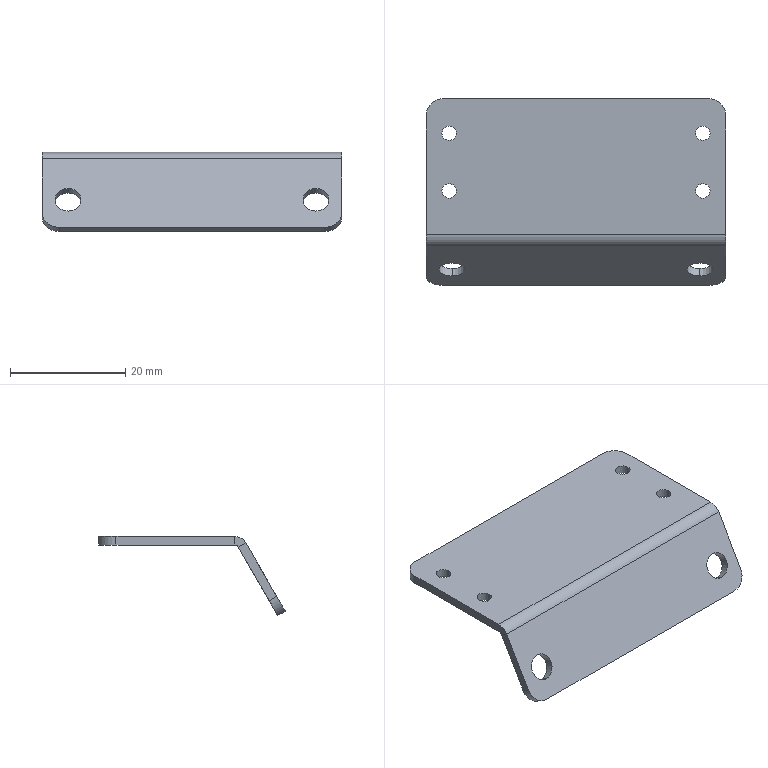Part | STEP file | 06-01-09 light source inclined plate (Default) | 1 solid | 30 faces | box 52 x 32.366 x 13.74 mm | volume 2941 mm3 | cylinder 18 | plane 12 | commonest cylinder face diameters 2.5 x8 4.5 x4 6 x4 1.473 x1 4.473 x1
STEP:
#1=CARTESIAN_POINT('',(21.5,-16.491,-6.279));
#2=VERTEX_POINT('',#1);
#3=CARTESIAN_POINT('',(21.5,-18.741,-10.176));
#4=VERTEX_POINT('',#3);
#5=CARTESIAN_POINT('',(21.5,-17.616,-8.227));
#6=DIRECTION('',(0.,-0.866,0.5));
#7=DIRECTION('',(0.,-0.5,-0.866));
#8=AXIS2_PLACEMENT_3D('',#5,#6,#7);
#9=CIRCLE('',#8,2.25);
#10=EDGE_CURVE('',#2,#4,#9,.T.);
#11=ORIENTED_EDGE('',*,*,#10,.T.);
#12=CARTESIAN_POINT('',(21.5,-17.442,-10.926));
#13=VERTEX_POINT('',#12);
#14=CARTESIAN_POINT('',(21.5,-26.102,-5.926));
#15=DIRECTION('',(0.,0.866,-0.5));
#16=VECTOR('',#15,1000.);
#17=LINE('',#14,#16);
#18=EDGE_CURVE('',#4,#13,#17,.T.);
#19=ORIENTED_EDGE('',*,*,#18,.T.);
#20=CARTESIAN_POINT('',(21.5,-15.192,-7.029));
#21=VERTEX_POINT('',#20);
#22=CARTESIAN_POINT('',(21.5,-16.317,-8.977));
#23=DIRECTION('',(0.,0.866,-0.5));
#24=DIRECTION('',(0.,0.5,0.866));
#25=AXIS2_PLACEMENT_3D('',#22,#23,#24);
#26=CIRCLE('',#25,2.25);
#27=EDGE_CURVE('',#13,#21,#26,.T.);
#28=ORIENTED_EDGE('',*,*,#27,.T.);
#29=CARTESIAN_POINT('',(21.5,-23.852,-2.029));
#30=DIRECTION('',(0.,0.866,-0.5));
#31=VECTOR('',#30,1000.);
#32=LINE('',#29,#31);
#33=EDGE_CURVE('',#2,#21,#32,.T.);
#34=ORIENTED_EDGE('',*,*,#33,.F.);
#35=EDGE_LOOP('',(#11,#19,#28,#34));
#36=FACE_OUTER_BOUND('',#35,.T.);
#37=CARTESIAN_POINT('',(21.5,-24.977,-3.977));
#38=DIRECTION('',(0.,0.866,-0.5));
#39=DIRECTION('',(0.,0.5,0.866));
#40=AXIS2_PLACEMENT_3D('',#37,#38,#39);
#41=CYLINDRICAL_SURFACE('',#40,2.25);
#42=ADVANCED_FACE('',(#36),#41,.F.);
#43=CARTESIAN_POINT('',(-21.5,-16.491,-6.279));
#44=VERTEX_POINT('',#43);
#45=CARTESIAN_POINT('',(-21.5,-18.741,-10.176));
#46=VERTEX_POINT('',#45);
#47=CARTESIAN_POINT('',(-21.5,-17.616,-8.227));
#48=DIRECTION('',(0.,-0.866,0.5));
#49=DIRECTION('',(0.,-0.5,-0.866));
#50=AXIS2_PLACEMENT_3D('',#47,#48,#49);
#51=CIRCLE('',#50,2.25);
#52=EDGE_CURVE('',#44,#46,#51,.T.);
#53=ORIENTED_EDGE('',*,*,#52,.T.);
#54=CARTESIAN_POINT('',(-21.5,-17.442,-10.926));
#55=VERTEX_POINT('',#54);
#56=CARTESIAN_POINT('',(-21.5,-26.102,-5.926));
#57=DIRECTION('',(0.,0.866,-0.5));
#58=VECTOR('',#57,1000.);
#59=LINE('',#56,#58);
#60=EDGE_CURVE('',#46,#55,#59,.T.);
#61=ORIENTED_EDGE('',*,*,#60,.T.);
#62=CARTESIAN_POINT('',(-21.5,-15.192,-7.029));
#63=VERTEX_POINT('',#62);
#64=CARTESIAN_POINT('',(-21.5,-16.317,-8.977));
#65=DIRECTION('',(0.,0.866,-0.5));
#66=DIRECTION('',(0.,0.5,0.866));
#67=AXIS2_PLACEMENT_3D('',#64,#65,#66);
#68=CIRCLE('',#67,2.25);
#69=EDGE_CURVE('',#55,#63,#68,.T.);
#70=ORIENTED_EDGE('',*,*,#69,.T.);
#71=CARTESIAN_POINT('',(-21.5,-23.852,-2.029));
#72=DIRECTION('',(0.,0.866,-0.5));
#73=VECTOR('',#72,1000.);
#74=LINE('',#71,#73);
#75=EDGE_CURVE('',#44,#63,#74,.T.);
#76=ORIENTED_EDGE('',*,*,#75,.F.);
#77=EDGE_LOOP('',(#53,#61,#70,#76));
#78=FACE_OUTER_BOUND('',#77,.T.);
#79=CARTESIAN_POINT('',(-21.5,-24.977,-3.977));
#80=DIRECTION('',(0.,0.866,-0.5));
#81=DIRECTION('',(0.,0.5,0.866));
#82=AXIS2_PLACEMENT_3D('',#79,#80,#81);
#83=CYLINDRICAL_SURFACE('',#82,2.25);
#84=ADVANCED_FACE('',(#78),#83,.F.);
#85=CARTESIAN_POINT('',(20.75,-4.,0.));
#86=VERTEX_POINT('',#85);
#87=CARTESIAN_POINT('',(23.25,-4.,0.));
#88=VERTEX_POINT('',#87);
#89=CARTESIAN_POINT('',(22.,-4.,0.));
#90=DIRECTION('',(0.,0.,1.));
#91=DIRECTION('',(1.,0.,0.));
#92=AXIS2_PLACEMENT_3D('',#89,#90,#91);
#93=CIRCLE('',#92,1.25);
#94=EDGE_CURVE('',#86,#88,#93,.T.);
#95=ORIENTED_EDGE('',*,*,#94,.T.);
#96=CARTESIAN_POINT('',(23.25,-4.,-1.5));
#97=VERTEX_POINT('',#96);
#98=CARTESIAN_POINT('',(23.25,-4.,-1.5));
#99=DIRECTION('',(0.,0.,-1.));
#100=VECTOR('',#99,1000.);
#101=LINE('',#98,#100);
#102=EDGE_CURVE('',#88,#97,#101,.T.);
#103=ORIENTED_EDGE('',*,*,#102,.T.);
#104=CARTESIAN_POINT('',(20.75,-4.,-1.5));
#105=VERTEX_POINT('',#104);
#106=CARTESIAN_POINT('',(22.,-4.,-1.5));
#107=DIRECTION('',(0.,0.,-1.));
#108=DIRECTION('',(-1.,0.,0.));
#109=AXIS2_PLACEMENT_3D('',#106,#107,#108);
#110=CIRCLE('',#109,1.25);
#111=EDGE_CURVE('',#97,#105,#110,.T.);
#112=ORIENTED_EDGE('',*,*,#111,.T.);
#113=CARTESIAN_POINT('',(20.75,-4.,-1.5));
#114=DIRECTION('',(0.,0.,-1.));
#115=VECTOR('',#114,1000.);
#116=LINE('',#113,#115);
#117=EDGE_CURVE('',#86,#105,#116,.T.);
#118=ORIENTED_EDGE('',*,*,#117,.F.);
#119=EDGE_LOOP('',(#95,#103,#112,#118));
#120=FACE_OUTER_BOUND('',#119,.T.);
#121=CARTESIAN_POINT('',(22.,-4.,-1.5));
#122=DIRECTION('',(0.,0.,-1.));
#123=DIRECTION('',(-1.,0.,0.));
#124=AXIS2_PLACEMENT_3D('',#121,#122,#123);
#125=CYLINDRICAL_SURFACE('',#124,1.25);
#126=ADVANCED_FACE('',(#120),#125,.F.);
#127=CARTESIAN_POINT('',(20.75,6.,0.));
#128=VERTEX_POINT('',#127);
#129=CARTESIAN_POINT('',(23.25,6.,0.));
#130=VERTEX_POINT('',#129);
#131=CARTESIAN_POINT('',(22.,6.,0.));
#132=DIRECTION('',(0.,0.,1.));
#133=DIRECTION('',(1.,0.,0.));
#134=AXIS2_PLACEMENT_3D('',#131,#132,#133);
#135=CIRCLE('',#134,1.25);
#136=EDGE_CURVE('',#128,#130,#135,.T.);
#137=ORIENTED_EDGE('',*,*,#136,.T.);
#138=CARTESIAN_POINT('',(23.25,6.,-1.5));
#139=VERTEX_POINT('',#138);
#140=CARTESIAN_POINT('',(23.25,6.,-1.5));
#141=DIRECTION('',(0.,0.,-1.));
#142=VECTOR('',#141,1000.);
#143=LINE('',#140,#142);
#144=EDGE_CURVE('',#130,#139,#143,.T.);
#145=ORIENTED_EDGE('',*,*,#144,.T.);
#146=CARTESIAN_POINT('',(20.75,6.,-1.5));
#147=VERTEX_POINT('',#146);
#148=CARTESIAN_POINT('',(22.,6.,-1.5));
#149=DIRECTION('',(0.,0.,-1.));
#150=DIRECTION('',(-1.,0.,0.));
#151=AXIS2_PLACEMENT_3D('',#148,#149,#150);
#152=CIRCLE('',#151,1.25);
#153=EDGE_CURVE('',#139,#147,#152,.T.);
#154=ORIENTED_EDGE('',*,*,#153,.T.);
#155=CARTESIAN_POINT('',(20.75,6.,-1.5));
#156=DIRECTION('',(0.,0.,-1.));
#157=VECTOR('',#156,1000.);
#158=LINE('',#155,#157);
#159=EDGE_CURVE('',#128,#147,#158,.T.);
#160=ORIENTED_EDGE('',*,*,#159,.F.);
#161=EDGE_LOOP('',(#137,#145,#154,#160));
#162=FACE_OUTER_BOUND('',#161,.T.);
#163=CARTESIAN_POINT('',(22.,6.,-1.5));
#164=DIRECTION('',(0.,0.,-1.));
#165=DIRECTION('',(-1.,0.,0.));
#166=AXIS2_PLACEMENT_3D('',#163,#164,#165);
#167=CYLINDRICAL_SURFACE('',#166,1.25);
#168=ADVANCED_FACE('',(#162),#167,.F.);
#169=CARTESIAN_POINT('',(-23.25,6.,0.));
#170=VERTEX_POINT('',#169);
#171=CARTESIAN_POINT('',(-20.75,6.,0.));
#172=VERTEX_POINT('',#171);
#173=CARTESIAN_POINT('',(-22.,6.,0.));
#174=DIRECTION('',(0.,0.,1.));
#175=DIRECTION('',(1.,0.,0.));
#176=AXIS2_PLACEMENT_3D('',#173,#174,#175);
#177=CIRCLE('',#176,1.25);
#178=EDGE_CURVE('',#170,#172,#177,.T.);
#179=ORIENTED_EDGE('',*,*,#178,.T.);
#180=CARTESIAN_POINT('',(-20.75,6.,-1.5));
#181=VERTEX_POINT('',#180);
#182=CARTESIAN_POINT('',(-20.75,6.,-1.5));
#183=DIRECTION('',(0.,0.,-1.));
#184=VECTOR('',#183,1000.);
#185=LINE('',#182,#184);
#186=EDGE_CURVE('',#172,#181,#185,.T.);
#187=ORIENTED_EDGE('',*,*,#186,.T.);
#188=CARTESIAN_POINT('',(-23.25,6.,-1.5));
#189=VERTEX_POINT('',#188);
#190=CARTESIAN_POINT('',(-22.,6.,-1.5));
#191=DIRECTION('',(0.,0.,-1.));
#192=DIRECTION('',(-1.,0.,0.));
#193=AXIS2_PLACEMENT_3D('',#190,#191,#192);
#194=CIRCLE('',#193,1.25);
#195=EDGE_CURVE('',#181,#189,#194,.T.);
#196=ORIENTED_EDGE('',*,*,#195,.T.);
#197=CARTESIAN_POINT('',(-23.25,6.,-1.5));
#198=DIRECTION('',(0.,0.,-1.));
#199=VECTOR('',#198,1000.);
#200=LINE('',#197,#199);
#201=EDGE_CURVE('',#170,#189,#200,.T.);
#202=ORIENTED_EDGE('',*,*,#201,.F.);
#203=EDGE_LOOP('',(#179,#187,#196,#202));
#204=FACE_OUTER_BOUND('',#203,.T.);
#205=CARTESIAN_POINT('',(-22.,6.,-1.5));
#206=DIRECTION('',(0.,0.,-1.));
#207=DIRECTION('',(-1.,0.,0.));
#208=AXIS2_PLACEMENT_3D('',#205,#206,#207);
#209=CYLINDRICAL_SURFACE('',#208,1.25);
#210=ADVANCED_FACE('',(#204),#209,.F.);
#211=CARTESIAN_POINT('',(-23.25,-4.,0.));
#212=VERTEX_POINT('',#211);
#213=CARTESIAN_POINT('',(-20.75,-4.,0.));
#214=VERTEX_POINT('',#213);
#215=CARTESIAN_POINT('',(-22.,-4.,0.));
#216=DIRECTION('',(0.,0.,1.));
#217=DIRECTION('',(1.,0.,0.));
#218=AXIS2_PLACEMENT_3D('',#215,#216,#217);
#219=CIRCLE('',#218,1.25);
#220=EDGE_CURVE('',#212,#214,#219,.T.);
#221=ORIENTED_EDGE('',*,*,#220,.T.);
#222=CARTESIAN_POINT('',(-20.75,-4.,-1.5));
#223=VERTEX_POINT('',#222);
#224=CARTESIAN_POINT('',(-20.75,-4.,-1.5));
#225=DIRECTION('',(0.,0.,-1.));
#226=VECTOR('',#225,1000.);
#227=LINE('',#224,#226);
#228=EDGE_CURVE('',#214,#223,#227,.T.);
#229=ORIENTED_EDGE('',*,*,#228,.T.);
#230=CARTESIAN_POINT('',(-23.25,-4.,-1.5));
#231=VERTEX_POINT('',#230);
#232=CARTESIAN_POINT('',(-22.,-4.,-1.5));
#233=DIRECTION('',(0.,0.,-1.));
#234=DIRECTION('',(-1.,0.,0.));
#235=AXIS2_PLACEMENT_3D('',#232,#233,#234);
#236=CIRCLE('',#235,1.25);
#237=EDGE_CURVE('',#223,#231,#236,.T.);
#238=ORIENTED_EDGE('',*,*,#237,.T.);
#239=CARTESIAN_POINT('',(-23.25,-4.,-1.5));
#240=DIRECTION('',(0.,0.,-1.));
#241=VECTOR('',#240,1000.);
#242=LINE('',#239,#241);
#243=EDGE_CURVE('',#212,#231,#242,.T.);
#244=ORIENTED_EDGE('',*,*,#243,.F.);
#245=EDGE_LOOP('',(#221,#229,#238,#244));
#246=FACE_OUTER_BOUND('',#245,.T.);
#247=CARTESIAN_POINT('',(-22.,-4.,-1.5));
#248=DIRECTION('',(0.,0.,-1.));
#249=DIRECTION('',(-1.,0.,0.));
#250=AXIS2_PLACEMENT_3D('',#247,#248,#249);
#251=CYLINDRICAL_SURFACE('',#250,1.25);
#252=ADVANCED_FACE('',(#246),#251,.F.);
#253=CARTESIAN_POINT('',(-26.,9.,0.));
#254=VERTEX_POINT('',#253);
#255=CARTESIAN_POINT('',(-26.,-11.575,0.));
#256=VERTEX_POINT('',#255);
#257=CARTESIAN_POINT('',(-26.,12.,0.));
#258=DIRECTION('',(0.,-1.,0.));
#259=VECTOR('',#258,1000.);
#260=LINE('',#257,#259);
#261=EDGE_CURVE('',#254,#256,#260,.T.);
#262=ORIENTED_EDGE('',*,*,#261,.F.);
#263=CARTESIAN_POINT('',(-26.,9.,-1.5));
#264=VERTEX_POINT('',#263);
#265=CARTESIAN_POINT('',(-26.,9.,-1.5));
#266=DIRECTION('',(0.,0.,-1.));
#267=VECTOR('',#266,1000.);
#268=LINE('',#265,#267);
#269=EDGE_CURVE('',#254,#264,#268,.T.);
#270=ORIENTED_EDGE('',*,*,#269,.T.);
#271=CARTESIAN_POINT('',(-26.,-11.575,-1.5));
#272=VERTEX_POINT('',#271);
#273=CARTESIAN_POINT('',(-26.,12.,-1.5));
#274=DIRECTION('',(0.,-1.,0.));
#275=VECTOR('',#274,1000.);
#276=LINE('',#273,#275);
#277=EDGE_CURVE('',#264,#272,#276,.T.);
#278=ORIENTED_EDGE('',*,*,#277,.T.);
#279=CARTESIAN_POINT('',(-26.,-11.575,-1.5));
#280=DIRECTION('',(0.,0.,1.));
#281=VECTOR('',#280,1000.);
#282=LINE('',#279,#281);
#283=EDGE_CURVE('',#272,#256,#282,.T.);
#284=ORIENTED_EDGE('',*,*,#283,.T.);
#285=EDGE_LOOP('',(#262,#270,#278,#284));
#286=FACE_OUTER_BOUND('',#285,.T.);
#287=CARTESIAN_POINT('',(-26.,12.,-1.5));
#288=DIRECTION('',(-1.,0.,0.));
#289=DIRECTION('',(0.,-1.,0.));
#290=AXIS2_PLACEMENT_3D('',#287,#288,#289);
#291=PLANE('',#290);
#292=ADVANCED_FACE('',(#286),#291,.T.);
#293=CARTESIAN_POINT('',(22.,-4.,-1.5));
#294=DIRECTION('',(0.,0.,-1.));
#295=DIRECTION('',(-1.,0.,0.));
#296=AXIS2_PLACEMENT_3D('',#293,#294,#295);
#297=CIRCLE('',#296,1.25);
#298=EDGE_CURVE('',#105,#97,#297,.T.);
#299=ORIENTED_EDGE('',*,*,#298,.F.);
#300=ORIENTED_EDGE('',*,*,#111,.F.);
#301=EDGE_LOOP('',(#299,#300));
#302=FACE_BOUND('',#301,.T.);
#303=CARTESIAN_POINT('',(22.,6.,-1.5));
#304=DIRECTION('',(0.,0.,-1.));
#305=DIRECTION('',(-1.,0.,0.));
#306=AXIS2_PLACEMENT_3D('',#303,#304,#305);
#307=CIRCLE('',#306,1.25);
#308=EDGE_CURVE('',#147,#139,#307,.T.);
#309=ORIENTED_EDGE('',*,*,#308,.F.);
#310=ORIENTED_EDGE('',*,*,#153,.F.);
#311=EDGE_LOOP('',(#309,#310));
#312=FACE_BOUND('',#311,.T.);
#313=CARTESIAN_POINT('',(-22.,6.,-1.5));
#314=DIRECTION('',(0.,0.,-1.));
#315=DIRECTION('',(-1.,0.,0.));
#316=AXIS2_PLACEMENT_3D('',#313,#314,#315);
#317=CIRCLE('',#316,1.25);
#318=EDGE_CURVE('',#189,#181,#317,.T.);
#319=ORIENTED_EDGE('',*,*,#318,.F.);
#320=ORIENTED_EDGE('',*,*,#195,.F.);
#321=EDGE_LOOP('',(#319,#320));
#322=FACE_BOUND('',#321,.T.);
#323=CARTESIAN_POINT('',(-22.,-4.,-1.5));
#324=DIRECTION('',(0.,0.,-1.));
#325=DIRECTION('',(-1.,0.,0.));
#326=AXIS2_PLACEMENT_3D('',#323,#324,#325);
#327=CIRCLE('',#326,1.25);
#328=EDGE_CURVE('',#231,#223,#327,.T.);
#329=ORIENTED_EDGE('',*,*,#328,.F.);
#330=ORIENTED_EDGE('',*,*,#237,.F.);
#331=EDGE_LOOP('',(#329,#330));
#332=FACE_BOUND('',#331,.T.);
#333=ORIENTED_EDGE('',*,*,#277,.F.);
#334=CARTESIAN_POINT('',(-23.,12.,-1.5));
#335=VERTEX_POINT('',#334);
#336=CARTESIAN_POINT('',(-23.,9.,-1.5));
#337=DIRECTION('',(0.,0.,-1.));
#338=DIRECTION('',(1.,0.,0.));
#339=AXIS2_PLACEMENT_3D('',#336,#337,#338);
#340=CIRCLE('',#339,3.);
#341=EDGE_CURVE('',#264,#335,#340,.T.);
#342=ORIENTED_EDGE('',*,*,#341,.T.);
#343=CARTESIAN_POINT('',(23.,12.,-1.5));
#344=VERTEX_POINT('',#343);
#345=CARTESIAN_POINT('',(-26.,12.,-1.5));
#346=DIRECTION('',(-1.,0.,0.));
#347=VECTOR('',#346,1000.);
#348=LINE('',#345,#347);
#349=EDGE_CURVE('',#344,#335,#348,.T.);
#350=ORIENTED_EDGE('',*,*,#349,.F.);
#351=CARTESIAN_POINT('',(26.,9.,-1.5));
#352=VERTEX_POINT('',#351);
#353=CARTESIAN_POINT('',(23.,9.,-1.5));
#354=DIRECTION('',(0.,0.,-1.));
#355=DIRECTION('',(1.,0.,0.));
#356=AXIS2_PLACEMENT_3D('',#353,#354,#355);
#357=CIRCLE('',#356,3.);
#358=EDGE_CURVE('',#344,#352,#357,.T.);
#359=ORIENTED_EDGE('',*,*,#358,.T.);
#360=CARTESIAN_POINT('',(26.,-11.575,-1.5));
#361=VERTEX_POINT('',#360);
#362=CARTESIAN_POINT('',(26.,12.,-1.5));
#363=DIRECTION('',(0.,1.,0.));
#364=VECTOR('',#363,1000.);
#365=LINE('',#362,#364);
#366=EDGE_CURVE('',#361,#352,#365,.T.);
#367=ORIENTED_EDGE('',*,*,#366,.F.);
#368=CARTESIAN_POINT('',(-26.,-11.575,-1.5));
#369=DIRECTION('',(1.,0.,0.));
#370=VECTOR('',#369,1000.);
#371=LINE('',#368,#370);
#372=EDGE_CURVE('',#272,#361,#371,.T.);
#373=ORIENTED_EDGE('',*,*,#372,.F.);
#374=EDGE_LOOP('',(#333,#342,#350,#359,#367,#373));
#375=FACE_OUTER_BOUND('',#374,.T.);
#376=CARTESIAN_POINT('',(26.,-12.,-1.5));
#377=DIRECTION('',(0.,0.,1.));
#378=DIRECTION('',(1.,0.,0.));
#379=AXIS2_PLACEMENT_3D('',#376,#377,#378);
#380=PLANE('',#379);
#381=ADVANCED_FACE('',(#302,#312,#322,#332,#375),#380,.F.);
#382=ORIENTED_EDGE('',*,*,#94,.F.);
#383=CARTESIAN_POINT('',(22.,-4.,0.));
#384=DIRECTION('',(0.,0.,1.));
#385=DIRECTION('',(1.,0.,0.));
#386=AXIS2_PLACEMENT_3D('',#383,#384,#385);
#387=CIRCLE('',#386,1.25);
#388=EDGE_CURVE('',#88,#86,#387,.T.);
#389=ORIENTED_EDGE('',*,*,#388,.F.);
#390=EDGE_LOOP('',(#382,#389));
#391=FACE_BOUND('',#390,.T.);
#392=ORIENTED_EDGE('',*,*,#136,.F.);
#393=CARTESIAN_POINT('',(22.,6.,0.));
#394=DIRECTION('',(0.,0.,1.));
#395=DIRECTION('',(1.,0.,0.));
#396=AXIS2_PLACEMENT_3D('',#393,#394,#395);
#397=CIRCLE('',#396,1.25);
#398=EDGE_CURVE('',#130,#128,#397,.T.);
#399=ORIENTED_EDGE('',*,*,#398,.F.);
#400=EDGE_LOOP('',(#392,#399));
#401=FACE_BOUND('',#400,.T.);
#402=ORIENTED_EDGE('',*,*,#178,.F.);
#403=CARTESIAN_POINT('',(-22.,6.,0.));
#404=DIRECTION('',(0.,0.,1.));
#405=DIRECTION('',(1.,0.,0.));
#406=AXIS2_PLACEMENT_3D('',#403,#404,#405);
#407=CIRCLE('',#406,1.25);
#408=EDGE_CURVE('',#172,#170,#407,.T.);
#409=ORIENTED_EDGE('',*,*,#408,.F.);
#410=EDGE_LOOP('',(#402,#409));
#411=FACE_BOUND('',#410,.T.);
#412=ORIENTED_EDGE('',*,*,#220,.F.);
#413=CARTESIAN_POINT('',(-22.,-4.,0.));
#414=DIRECTION('',(0.,0.,1.));
#415=DIRECTION('',(1.,0.,0.));
#416=AXIS2_PLACEMENT_3D('',#413,#414,#415);
#417=CIRCLE('',#416,1.25);
#418=EDGE_CURVE('',#214,#212,#417,.T.);
#419=ORIENTED_EDGE('',*,*,#418,.F.);
#420=EDGE_LOOP('',(#412,#419));
#421=FACE_BOUND('',#420,.T.);
#422=CARTESIAN_POINT('',(23.,12.,0.));
#423=VERTEX_POINT('',#422);
#424=CARTESIAN_POINT('',(-23.,12.,0.));
#425=VERTEX_POINT('',#424);
#426=CARTESIAN_POINT('',(-26.,12.,0.));
#427=DIRECTION('',(-1.,0.,0.));
#428=VECTOR('',#427,1000.);
#429=LINE('',#426,#428);
#430=EDGE_CURVE('',#423,#425,#429,.T.);
#431=ORIENTED_EDGE('',*,*,#430,.T.);
#432=CARTESIAN_POINT('',(-23.,9.,0.));
#433=DIRECTION('',(0.,0.,1.));
#434=DIRECTION('',(1.,0.,0.));
#435=AXIS2_PLACEMENT_3D('',#432,#433,#434);
#436=CIRCLE('',#435,3.);
#437=EDGE_CURVE('',#425,#254,#436,.T.);
#438=ORIENTED_EDGE('',*,*,#437,.T.);
#439=ORIENTED_EDGE('',*,*,#261,.T.);
#440=CARTESIAN_POINT('',(26.,-11.575,0.));
#441=VERTEX_POINT('',#440);
#442=CARTESIAN_POINT('',(-26.,-11.575,0.));
#443=DIRECTION('',(1.,0.,0.));
#444=VECTOR('',#443,1000.);
#445=LINE('',#442,#444);
#446=EDGE_CURVE('',#256,#441,#445,.T.);
#447=ORIENTED_EDGE('',*,*,#446,.T.);
#448=CARTESIAN_POINT('',(26.,9.,0.));
#449=VERTEX_POINT('',#448);
#450=CARTESIAN_POINT('',(26.,12.,0.));
#451=DIRECTION('',(0.,1.,0.));
#452=VECTOR('',#451,1000.);
#453=LINE('',#450,#452);
#454=EDGE_CURVE('',#441,#449,#453,.T.);
#455=ORIENTED_EDGE('',*,*,#454,.T.);
#456=CARTESIAN_POINT('',(23.,9.,0.));
#457=DIRECTION('',(0.,0.,1.));
#458=DIRECTION('',(1.,0.,0.));
#459=AXIS2_PLACEMENT_3D('',#456,#457,#458);
#460=CIRCLE('',#459,3.);
#461=EDGE_CURVE('',#449,#423,#460,.T.);
#462=ORIENTED_EDGE('',*,*,#461,.T.);
#463=EDGE_LOOP('',(#431,#438,#439,#447,#455,#462));
#464=FACE_OUTER_BOUND('',#463,.T.);
#465=CARTESIAN_POINT('',(26.,-12.,0.));
#466=DIRECTION('',(0.,0.,1.));
#467=DIRECTION('',(1.,0.,0.));
#468=AXIS2_PLACEMENT_3D('',#465,#466,#467);
#469=PLANE('',#468);
#470=ADVANCED_FACE('',(#391,#401,#411,#421,#464),#469,.T.);
#471=ORIENTED_EDGE('',*,*,#366,.T.);
#472=CARTESIAN_POINT('',(26.,9.,-1.5));
#473=DIRECTION('',(0.,0.,1.));
#474=VECTOR('',#473,1000.);
#475=LINE('',#472,#474);
#476=EDGE_CURVE('',#352,#449,#475,.T.);
#477=ORIENTED_EDGE('',*,*,#476,.T.);
#478=ORIENTED_EDGE('',*,*,#454,.F.);
#479=CARTESIAN_POINT('',(26.,-11.575,-1.5));
#480=DIRECTION('',(0.,0.,1.));
#481=VECTOR('',#480,1000.);
#482=LINE('',#479,#481);
#483=EDGE_CURVE('',#361,#441,#482,.T.);
#484=ORIENTED_EDGE('',*,*,#483,.F.);
#485=EDGE_LOOP('',(#471,#477,#478,#484));
#486=FACE_OUTER_BOUND('',#485,.T.);
#487=CARTESIAN_POINT('',(26.,12.,-1.5));
#488=DIRECTION('',(1.,0.,0.));
#489=DIRECTION('',(0.,0.,-1.));
#490=AXIS2_PLACEMENT_3D('',#487,#488,#489);
#491=PLANE('',#490);
#492=ADVANCED_FACE('',(#486),#491,.T.);
#493=ORIENTED_EDGE('',*,*,#349,.T.);
#494=CARTESIAN_POINT('',(-23.,12.,-1.5));
#495=DIRECTION('',(0.,0.,1.));
#496=VECTOR('',#495,1000.);
#497=LINE('',#494,#496);
#498=EDGE_CURVE('',#335,#425,#497,.T.);
#499=ORIENTED_EDGE('',*,*,#498,.T.);
#500=ORIENTED_EDGE('',*,*,#430,.F.);
#501=CARTESIAN_POINT('',(23.,12.,-1.5));
#502=DIRECTION('',(0.,0.,-1.));
#503=VECTOR('',#502,1000.);
#504=LINE('',#501,#503);
#505=EDGE_CURVE('',#423,#344,#504,.T.);
#506=ORIENTED_EDGE('',*,*,#505,.T.);
#507=EDGE_LOOP('',(#493,#499,#500,#506));
#508=FACE_OUTER_BOUND('',#507,.T.);
#509=CARTESIAN_POINT('',(-26.,12.,-1.5));
#510=DIRECTION('',(0.,1.,0.));
#511=DIRECTION('',(0.,0.,1.));
#512=AXIS2_PLACEMENT_3D('',#509,#510,#511);
#513=PLANE('',#512);
#514=ADVANCED_FACE('',(#508),#513,.T.);
#515=CARTESIAN_POINT('',(26.,-12.213,-1.868));
#516=VERTEX_POINT('',#515);
#517=CARTESIAN_POINT('',(26.,-13.512,-1.118));
#518=VERTEX_POINT('',#517);
#519=CARTESIAN_POINT('',(26.,-12.213,-1.868));
#520=DIRECTION('',(0.,-0.866,0.5));
#521=VECTOR('',#520,1000.);
#522=LINE('',#519,#521);
#523=EDGE_CURVE('',#516,#518,#522,.T.);
#524=ORIENTED_EDGE('',*,*,#523,.F.);
#525=CARTESIAN_POINT('',(26.,-11.575,-2.237));
#526=DIRECTION('',(1.,0.,0.));
#527=DIRECTION('',(0.,0.,1.));
#528=AXIS2_PLACEMENT_3D('',#525,#526,#527);
#529=CIRCLE('',#528,0.7366);
#530=EDGE_CURVE('',#361,#516,#529,.T.);
#531=ORIENTED_EDGE('',*,*,#530,.F.);
#532=ORIENTED_EDGE('',*,*,#483,.T.);
#533=CARTESIAN_POINT('',(26.,-11.575,-2.237));
#534=DIRECTION('',(1.,0.,0.));
#535=DIRECTION('',(0.,0.,1.));
#536=AXIS2_PLACEMENT_3D('',#533,#534,#535);
#537=CIRCLE('',#536,2.237);
#538=EDGE_CURVE('',#441,#518,#537,.T.);
#539=ORIENTED_EDGE('',*,*,#538,.T.);
#540=EDGE_LOOP('',(#524,#531,#532,#539));
#541=FACE_OUTER_BOUND('',#540,.T.);
#542=CARTESIAN_POINT('',(26.,-11.575,-2.237));
#543=DIRECTION('',(1.,0.,0.));
#544=DIRECTION('',(0.,0.,-1.));
#545=AXIS2_PLACEMENT_3D('',#542,#543,#544);
#546=PLANE('',#545);
#547=ADVANCED_FACE('',(#541),#546,.T.);
#548=CARTESIAN_POINT('',(-26.,-12.213,-1.868));
#549=VERTEX_POINT('',#548);
#550=CARTESIAN_POINT('',(-26.,-11.575,-2.237));
#551=DIRECTION('',(-1.,0.,0.));
#552=DIRECTION('',(0.,0.,1.));
#553=AXIS2_PLACEMENT_3D('',#550,#551,#552);
#554=CIRCLE('',#553,0.7366);
#555=EDGE_CURVE('',#549,#272,#554,.T.);
#556=ORIENTED_EDGE('',*,*,#555,.F.);
#557=CARTESIAN_POINT('',(-26.,-13.512,-1.118));
#558=VERTEX_POINT('',#557);
#559=CARTESIAN_POINT('',(-26.,-12.213,-1.868));
#560=DIRECTION('',(0.,-0.866,0.5));
#561=VECTOR('',#560,1000.);
#562=LINE('',#559,#561);
#563=EDGE_CURVE('',#549,#558,#562,.T.);
#564=ORIENTED_EDGE('',*,*,#563,.T.);
#565=CARTESIAN_POINT('',(-26.,-11.575,-2.237));
#566=DIRECTION('',(-1.,0.,0.));
#567=DIRECTION('',(0.,0.,1.));
#568=AXIS2_PLACEMENT_3D('',#565,#566,#567);
#569=CIRCLE('',#568,2.237);
#570=EDGE_CURVE('',#558,#256,#569,.T.);
#571=ORIENTED_EDGE('',*,*,#570,.T.);
#572=ORIENTED_EDGE('',*,*,#283,.F.);
#573=EDGE_LOOP('',(#556,#564,#571,#572));
#574=FACE_OUTER_BOUND('',#573,.T.);
#575=CARTESIAN_POINT('',(-26.,-11.575,-2.237));
#576=DIRECTION('',(1.,0.,0.));
#577=DIRECTION('',(0.,0.,-1.));
#578=AXIS2_PLACEMENT_3D('',#575,#576,#577);
#579=PLANE('',#578);
#580=ADVANCED_FACE('',(#574),#579,.F.);
#581=ORIENTED_EDGE('',*,*,#446,.F.);
#582=ORIENTED_EDGE('',*,*,#570,.F.);
#583=CARTESIAN_POINT('',(-26.,-13.512,-1.118));
#584=DIRECTION('',(-1.,0.,0.));
#585=VECTOR('',#584,1000.);
#586=LINE('',#583,#585);
#587=EDGE_CURVE('',#518,#558,#586,.T.);
#588=ORIENTED_EDGE('',*,*,#587,.F.);
#589=ORIENTED_EDGE('',*,*,#538,.F.);
#590=EDGE_LOOP('',(#581,#582,#588,#589));
#591=FACE_OUTER_BOUND('',#590,.T.);
#592=CARTESIAN_POINT('',(-26.,-11.575,-2.237));
#593=DIRECTION('',(-1.,0.,0.));
#594=DIRECTION('',(0.,-0.866,0.5));
#595=AXIS2_PLACEMENT_3D('',#592,#593,#594);
#596=CYLINDRICAL_SURFACE('',#595,2.237);
#597=ADVANCED_FACE('',(#591),#596,.T.);
#598=ORIENTED_EDGE('',*,*,#372,.T.);
#599=ORIENTED_EDGE('',*,*,#530,.T.);
#600=CARTESIAN_POINT('',(26.,-12.213,-1.868));
#601=DIRECTION('',(-1.,0.,0.));
#602=VECTOR('',#601,1000.);
#603=LINE('',#600,#602);
#604=EDGE_CURVE('',#516,#549,#603,.T.);
#605=ORIENTED_EDGE('',*,*,#604,.T.);
#606=ORIENTED_EDGE('',*,*,#555,.T.);
#607=EDGE_LOOP('',(#598,#599,#605,#606));
#608=FACE_OUTER_BOUND('',#607,.T.);
#609=CARTESIAN_POINT('',(-26.,-11.575,-2.237));
#610=DIRECTION('',(-1.,0.,0.));
#611=DIRECTION('',(0.,-0.866,0.5));
#612=AXIS2_PLACEMENT_3D('',#609,#610,#611);
#613=CYLINDRICAL_SURFACE('',#612,0.7366);
#614=ADVANCED_FACE('',(#608),#613,.F.);
#615=CARTESIAN_POINT('',(-26.,-17.567,-11.142));
#616=VERTEX_POINT('',#615);
#617=CARTESIAN_POINT('',(-26.,-12.,-1.5));
#618=DIRECTION('',(0.,0.5,0.866));
#619=VECTOR('',#618,1000.);
#620=LINE('',#617,#619);
#621=EDGE_CURVE('',#616,#549,#620,.T.);
#622=ORIENTED_EDGE('',*,*,#621,.F.);
#623=CARTESIAN_POINT('',(-26.,-18.866,-10.392));
#624=VERTEX_POINT('',#623);
#625=CARTESIAN_POINT('',(-26.,-18.866,-10.392));
#626=DIRECTION('',(0.,-0.866,0.5));
#627=VECTOR('',#626,1000.);
#628=LINE('',#625,#627);
#629=EDGE_CURVE('',#616,#624,#628,.T.);
#630=ORIENTED_EDGE('',*,*,#629,.T.);
#631=CARTESIAN_POINT('',(-26.,-13.299,-0.75));
#632=DIRECTION('',(0.,0.5,0.866));
#633=VECTOR('',#632,1000.);
#634=LINE('',#631,#633);
#635=EDGE_CURVE('',#624,#558,#634,.T.);
#636=ORIENTED_EDGE('',*,*,#635,.T.);
#637=ORIENTED_EDGE('',*,*,#563,.F.);
#638=EDGE_LOOP('',(#622,#630,#636,#637));
#639=FACE_OUTER_BOUND('',#638,.T.);
#640=CARTESIAN_POINT('',(-26.,-13.299,-0.75));
#641=DIRECTION('',(-1.,0.,0.));
#642=DIRECTION('',(0.,0.,1.));
#643=AXIS2_PLACEMENT_3D('',#640,#641,#642);
#644=PLANE('',#643);
#645=ADVANCED_FACE('',(#639),#644,.T.);
#646=CARTESIAN_POINT('',(26.,-18.866,-10.392));
#647=VERTEX_POINT('',#646);
#648=CARTESIAN_POINT('',(26.,-20.366,-12.99));
#649=DIRECTION('',(0.,-0.5,-0.866));
#650=VECTOR('',#649,1000.);
#651=LINE('',#648,#650);
#652=EDGE_CURVE('',#518,#647,#651,.T.);
#653=ORIENTED_EDGE('',*,*,#652,.T.);
#654=CARTESIAN_POINT('',(26.,-17.567,-11.142));
#655=VERTEX_POINT('',#654);
#656=CARTESIAN_POINT('',(26.,-18.866,-10.392));
#657=DIRECTION('',(0.,0.866,-0.5));
#658=VECTOR('',#657,1000.);
#659=LINE('',#656,#658);
#660=EDGE_CURVE('',#647,#655,#659,.T.);
#661=ORIENTED_EDGE('',*,*,#660,.T.);
#662=CARTESIAN_POINT('',(26.,-19.067,-13.74));
#663=DIRECTION('',(0.,-0.5,-0.866));
#664=VECTOR('',#663,1000.);
#665=LINE('',#662,#664);
#666=EDGE_CURVE('',#516,#655,#665,.T.);
#667=ORIENTED_EDGE('',*,*,#666,.F.);
#668=ORIENTED_EDGE('',*,*,#523,.T.);
#669=EDGE_LOOP('',(#653,#661,#667,#668));
#670=FACE_OUTER_BOUND('',#669,.T.);
#671=CARTESIAN_POINT('',(26.,-20.366,-12.99));
#672=DIRECTION('',(1.,0.,0.));
#673=DIRECTION('',(0.,0.,-1.));
#674=AXIS2_PLACEMENT_3D('',#671,#672,#673);
#675=PLANE('',#674);
#676=ADVANCED_FACE('',(#670),#675,.T.);
#677=ORIENTED_EDGE('',*,*,#10,.F.);
#678=CARTESIAN_POINT('',(21.5,-17.616,-8.227));
#679=DIRECTION('',(0.,-0.866,0.5));
#680=DIRECTION('',(0.,-0.5,-0.866));
#681=AXIS2_PLACEMENT_3D('',#678,#679,#680);
#682=CIRCLE('',#681,2.25);
#683=EDGE_CURVE('',#4,#2,#682,.T.);
#684=ORIENTED_EDGE('',*,*,#683,.F.);
#685=EDGE_LOOP('',(#677,#684));
#686=FACE_BOUND('',#685,.T.);
#687=ORIENTED_EDGE('',*,*,#52,.F.);
#688=CARTESIAN_POINT('',(-21.5,-17.616,-8.227));
#689=DIRECTION('',(0.,-0.866,0.5));
#690=DIRECTION('',(0.,-0.5,-0.866));
#691=AXIS2_PLACEMENT_3D('',#688,#689,#690);
#692=CIRCLE('',#691,2.25);
#693=EDGE_CURVE('',#46,#44,#692,.T.);
#694=ORIENTED_EDGE('',*,*,#693,.F.);
#695=EDGE_LOOP('',(#687,#694));
#696=FACE_BOUND('',#695,.T.);
#697=ORIENTED_EDGE('',*,*,#635,.F.);
#698=CARTESIAN_POINT('',(-23.,-20.366,-12.99));
#699=VERTEX_POINT('',#698);
#700=CARTESIAN_POINT('',(-23.,-18.866,-10.392));
#701=DIRECTION('',(0.,-0.866,0.5));
#702=DIRECTION('',(0.,-0.5,-0.866));
#703=AXIS2_PLACEMENT_3D('',#700,#701,#702);
#704=CIRCLE('',#703,3.);
#705=EDGE_CURVE('',#624,#699,#704,.T.);
#706=ORIENTED_EDGE('',*,*,#705,.T.);
#707=CARTESIAN_POINT('',(23.,-20.366,-12.99));
#708=VERTEX_POINT('',#707);
#709=CARTESIAN_POINT('',(-26.,-20.366,-12.99));
#710=DIRECTION('',(-1.,0.,0.));
#711=VECTOR('',#710,1000.);
#712=LINE('',#709,#711);
#713=EDGE_CURVE('',#708,#699,#712,.T.);
#714=ORIENTED_EDGE('',*,*,#713,.F.);
#715=CARTESIAN_POINT('',(23.,-18.866,-10.392));
#716=DIRECTION('',(0.,-0.866,0.5));
#717=DIRECTION('',(0.,-0.5,-0.866));
#718=AXIS2_PLACEMENT_3D('',#715,#716,#717);
#719=CIRCLE('',#718,3.);
#720=EDGE_CURVE('',#708,#647,#719,.T.);
#721=ORIENTED_EDGE('',*,*,#720,.T.);
#722=ORIENTED_EDGE('',*,*,#652,.F.);
#723=ORIENTED_EDGE('',*,*,#587,.T.);
#724=EDGE_LOOP('',(#697,#706,#714,#721,#722,#723));
#725=FACE_OUTER_BOUND('',#724,.T.);
#726=CARTESIAN_POINT('',(-26.,-13.299,-0.75));
#727=DIRECTION('',(0.,-0.866,0.5));
#728=DIRECTION('',(0.,-0.5,-0.866));
#729=AXIS2_PLACEMENT_3D('',#726,#727,#728);
#730=PLANE('',#729);
#731=ADVANCED_FACE('',(#686,#696,#725),#730,.T.);
#732=CARTESIAN_POINT('',(21.5,-16.317,-8.977));
#733=DIRECTION('',(0.,0.866,-0.5));
#734=DIRECTION('',(0.,0.5,0.866));
#735=AXIS2_PLACEMENT_3D('',#732,#733,#734);
#736=CIRCLE('',#735,2.25);
#737=EDGE_CURVE('',#21,#13,#736,.T.);
#738=ORIENTED_EDGE('',*,*,#737,.F.);
#739=ORIENTED_EDGE('',*,*,#27,.F.);
#740=EDGE_LOOP('',(#738,#739));
#741=FACE_BOUND('',#740,.T.);
#742=CARTESIAN_POINT('',(-21.5,-16.317,-8.977));
#743=DIRECTION('',(0.,0.866,-0.5));
#744=DIRECTION('',(0.,0.5,0.866));
#745=AXIS2_PLACEMENT_3D('',#742,#743,#744);
#746=CIRCLE('',#745,2.25);
#747=EDGE_CURVE('',#63,#55,#746,.T.);
#748=ORIENTED_EDGE('',*,*,#747,.F.);
#749=ORIENTED_EDGE('',*,*,#69,.F.);
#750=EDGE_LOOP('',(#748,#749));
#751=FACE_BOUND('',#750,.T.);
#752=CARTESIAN_POINT('',(23.,-19.067,-13.74));
#753=VERTEX_POINT('',#752);
#754=CARTESIAN_POINT('',(-23.,-19.067,-13.74));
#755=VERTEX_POINT('',#754);
#756=CARTESIAN_POINT('',(-26.,-19.067,-13.74));
#757=DIRECTION('',(-1.,0.,0.));
#758=VECTOR('',#757,1000.);
#759=LINE('',#756,#758);
#760=EDGE_CURVE('',#753,#755,#759,.T.);
#761=ORIENTED_EDGE('',*,*,#760,.T.);
#762=CARTESIAN_POINT('',(-23.,-17.567,-11.142));
#763=DIRECTION('',(0.,0.866,-0.5));
#764=DIRECTION('',(0.,-0.5,-0.866));
#765=AXIS2_PLACEMENT_3D('',#762,#763,#764);
#766=CIRCLE('',#765,3.);
#767=EDGE_CURVE('',#755,#616,#766,.T.);
#768=ORIENTED_EDGE('',*,*,#767,.T.);
#769=ORIENTED_EDGE('',*,*,#621,.T.);
#770=ORIENTED_EDGE('',*,*,#604,.F.);
#771=ORIENTED_EDGE('',*,*,#666,.T.);
#772=CARTESIAN_POINT('',(23.,-17.567,-11.142));
#773=DIRECTION('',(0.,0.866,-0.5));
#774=DIRECTION('',(0.,-0.5,-0.866));
#775=AXIS2_PLACEMENT_3D('',#772,#773,#774);
#776=CIRCLE('',#775,3.);
#777=EDGE_CURVE('',#655,#753,#776,.T.);
#778=ORIENTED_EDGE('',*,*,#777,.T.);
#779=EDGE_LOOP('',(#761,#768,#769,#770,#771,#778));
#780=FACE_OUTER_BOUND('',#779,.T.);
#781=CARTESIAN_POINT('',(-26.,-12.,-1.5));
#782=DIRECTION('',(0.,-0.866,0.5));
#783=DIRECTION('',(0.,-0.5,-0.866));
#784=AXIS2_PLACEMENT_3D('',#781,#782,#783);
#785=PLANE('',#784);
#786=ADVANCED_FACE('',(#741,#751,#780),#785,.F.);
#787=ORIENTED_EDGE('',*,*,#713,.T.);
#788=CARTESIAN_POINT('',(-23.,-20.366,-12.99));
#789=DIRECTION('',(0.,0.866,-0.5));
#790=VECTOR('',#789,1000.);
#791=LINE('',#788,#790);
#792=EDGE_CURVE('',#699,#755,#791,.T.);
#793=ORIENTED_EDGE('',*,*,#792,.T.);
#794=ORIENTED_EDGE('',*,*,#760,.F.);
#795=CARTESIAN_POINT('',(23.,-20.366,-12.99));
#796=DIRECTION('',(0.,-0.866,0.5));
#797=VECTOR('',#796,1000.);
#798=LINE('',#795,#797);
#799=EDGE_CURVE('',#753,#708,#798,.T.);
#800=ORIENTED_EDGE('',*,*,#799,.T.);
#801=EDGE_LOOP('',(#787,#793,#794,#800));
#802=FACE_OUTER_BOUND('',#801,.T.);
#803=CARTESIAN_POINT('',(-26.,-20.366,-12.99));
#804=DIRECTION('',(0.,-0.5,-0.866));
#805=DIRECTION('',(0.,0.866,-0.5));
#806=AXIS2_PLACEMENT_3D('',#803,#804,#805);
#807=PLANE('',#806);
#808=ADVANCED_FACE('',(#802),#807,.T.);
#809=ORIENTED_EDGE('',*,*,#228,.F.);
#810=ORIENTED_EDGE('',*,*,#418,.T.);
#811=ORIENTED_EDGE('',*,*,#243,.T.);
#812=ORIENTED_EDGE('',*,*,#328,.T.);
#813=EDGE_LOOP('',(#809,#810,#811,#812));
#814=FACE_OUTER_BOUND('',#813,.T.);
#815=CARTESIAN_POINT('',(-22.,-4.,-1.5));
#816=DIRECTION('',(0.,0.,-1.));
#817=DIRECTION('',(-1.,0.,0.));
#818=AXIS2_PLACEMENT_3D('',#815,#816,#817);
#819=CYLINDRICAL_SURFACE('',#818,1.25);
#820=ADVANCED_FACE('',(#814),#819,.F.);
#821=ORIENTED_EDGE('',*,*,#186,.F.);
#822=ORIENTED_EDGE('',*,*,#408,.T.);
#823=ORIENTED_EDGE('',*,*,#201,.T.);
#824=ORIENTED_EDGE('',*,*,#318,.T.);
#825=EDGE_LOOP('',(#821,#822,#823,#824));
#826=FACE_OUTER_BOUND('',#825,.T.);
#827=CARTESIAN_POINT('',(-22.,6.,-1.5));
#828=DIRECTION('',(0.,0.,-1.));
#829=DIRECTION('',(-1.,0.,0.));
#830=AXIS2_PLACEMENT_3D('',#827,#828,#829);
#831=CYLINDRICAL_SURFACE('',#830,1.25);
#832=ADVANCED_FACE('',(#826),#831,.F.);
#833=ORIENTED_EDGE('',*,*,#144,.F.);
#834=ORIENTED_EDGE('',*,*,#398,.T.);
#835=ORIENTED_EDGE('',*,*,#159,.T.);
#836=ORIENTED_EDGE('',*,*,#308,.T.);
#837=EDGE_LOOP('',(#833,#834,#835,#836));
#838=FACE_OUTER_BOUND('',#837,.T.);
#839=CARTESIAN_POINT('',(22.,6.,-1.5));
#840=DIRECTION('',(0.,0.,-1.));
#841=DIRECTION('',(-1.,0.,0.));
#842=AXIS2_PLACEMENT_3D('',#839,#840,#841);
#843=CYLINDRICAL_SURFACE('',#842,1.25);
#844=ADVANCED_FACE('',(#838),#843,.F.);
#845=ORIENTED_EDGE('',*,*,#102,.F.);
#846=ORIENTED_EDGE('',*,*,#388,.T.);
#847=ORIENTED_EDGE('',*,*,#117,.T.);
#848=ORIENTED_EDGE('',*,*,#298,.T.);
#849=EDGE_LOOP('',(#845,#846,#847,#848));
#850=FACE_OUTER_BOUND('',#849,.T.);
#851=CARTESIAN_POINT('',(22.,-4.,-1.5));
#852=DIRECTION('',(0.,0.,-1.));
#853=DIRECTION('',(-1.,0.,0.));
#854=AXIS2_PLACEMENT_3D('',#851,#852,#853);
#855=CYLINDRICAL_SURFACE('',#854,1.25);
#856=ADVANCED_FACE('',(#850),#855,.F.);
#857=ORIENTED_EDGE('',*,*,#705,.F.);
#858=ORIENTED_EDGE('',*,*,#629,.F.);
#859=ORIENTED_EDGE('',*,*,#767,.F.);
#860=ORIENTED_EDGE('',*,*,#792,.F.);
#861=EDGE_LOOP('',(#857,#858,#859,#860));
#862=FACE_OUTER_BOUND('',#861,.T.);
#863=CARTESIAN_POINT('',(-23.,-18.866,-10.392));
#864=DIRECTION('',(0.,0.866,-0.5));
#865=DIRECTION('',(0.,0.5,0.866));
#866=AXIS2_PLACEMENT_3D('',#863,#864,#865);
#867=CYLINDRICAL_SURFACE('',#866,3.);
#868=ADVANCED_FACE('',(#862),#867,.T.);
#869=ORIENTED_EDGE('',*,*,#341,.F.);
#870=ORIENTED_EDGE('',*,*,#269,.F.);
#871=ORIENTED_EDGE('',*,*,#437,.F.);
#872=ORIENTED_EDGE('',*,*,#498,.F.);
#873=EDGE_LOOP('',(#869,#870,#871,#872));
#874=FACE_OUTER_BOUND('',#873,.T.);
#875=CARTESIAN_POINT('',(-23.,9.,-1.5));
#876=DIRECTION('',(0.,0.,1.));
#877=DIRECTION('',(1.,0.,0.));
#878=AXIS2_PLACEMENT_3D('',#875,#876,#877);
#879=CYLINDRICAL_SURFACE('',#878,3.);
#880=ADVANCED_FACE('',(#874),#879,.T.);
#881=ORIENTED_EDGE('',*,*,#358,.F.);
#882=ORIENTED_EDGE('',*,*,#505,.F.);
#883=ORIENTED_EDGE('',*,*,#461,.F.);
#884=ORIENTED_EDGE('',*,*,#476,.F.);
#885=EDGE_LOOP('',(#881,#882,#883,#884));
#886=FACE_OUTER_BOUND('',#885,.T.);
#887=CARTESIAN_POINT('',(23.,9.,-1.5));
#888=DIRECTION('',(0.,0.,1.));
#889=DIRECTION('',(1.,0.,0.));
#890=AXIS2_PLACEMENT_3D('',#887,#888,#889);
#891=CYLINDRICAL_SURFACE('',#890,3.);
#892=ADVANCED_FACE('',(#886),#891,.T.);
#893=ORIENTED_EDGE('',*,*,#720,.F.);
#894=ORIENTED_EDGE('',*,*,#799,.F.);
#895=ORIENTED_EDGE('',*,*,#777,.F.);
#896=ORIENTED_EDGE('',*,*,#660,.F.);
#897=EDGE_LOOP('',(#893,#894,#895,#896));
#898=FACE_OUTER_BOUND('',#897,.T.);
#899=CARTESIAN_POINT('',(23.,-18.866,-10.392));
#900=DIRECTION('',(0.,0.866,-0.5));
#901=DIRECTION('',(0.,0.5,0.866));
#902=AXIS2_PLACEMENT_3D('',#899,#900,#901);
#903=CYLINDRICAL_SURFACE('',#902,3.);
#904=ADVANCED_FACE('',(#898),#903,.T.);
#905=ORIENTED_EDGE('',*,*,#60,.F.);
#906=ORIENTED_EDGE('',*,*,#693,.T.);
#907=ORIENTED_EDGE('',*,*,#75,.T.);
#908=ORIENTED_EDGE('',*,*,#747,.T.);
#909=EDGE_LOOP('',(#905,#906,#907,#908));
#910=FACE_OUTER_BOUND('',#909,.T.);
#911=CARTESIAN_POINT('',(-21.5,-24.977,-3.977));
#912=DIRECTION('',(0.,0.866,-0.5));
#913=DIRECTION('',(0.,0.5,0.866));
#914=AXIS2_PLACEMENT_3D('',#911,#912,#913);
#915=CYLINDRICAL_SURFACE('',#914,2.25);
#916=ADVANCED_FACE('',(#910),#915,.F.);
#917=ORIENTED_EDGE('',*,*,#18,.F.);
#918=ORIENTED_EDGE('',*,*,#683,.T.);
#919=ORIENTED_EDGE('',*,*,#33,.T.);
#920=ORIENTED_EDGE('',*,*,#737,.T.);
#921=EDGE_LOOP('',(#917,#918,#919,#920));
#922=FACE_OUTER_BOUND('',#921,.T.);
#923=CARTESIAN_POINT('',(21.5,-24.977,-3.977));
#924=DIRECTION('',(0.,0.866,-0.5));
#925=DIRECTION('',(0.,0.5,0.866));
#926=AXIS2_PLACEMENT_3D('',#923,#924,#925);
#927=CYLINDRICAL_SURFACE('',#926,2.25);
#928=ADVANCED_FACE('',(#922),#927,.F.);
#929=CLOSED_SHELL('',(#42,#84,#126,#168,#210,#252,#292,#381,#470,#492,#514,#547,#580,#597,#614,#645,#676,#731,#786,#808,#820,#832,#844,#856,#868,#880,#892,#904,#916,#928));
#930=MANIFOLD_SOLID_BREP('',#929);
#931=CARTESIAN_POINT('',(0.,0.,0.));
#932=DIRECTION('',(0.,0.,1.));
#933=DIRECTION('',(1.,0.,0.));
#934=AXIS2_PLACEMENT_3D('',#931,#932,#933);
#935=(LENGTH_UNIT()NAMED_UNIT(*)SI_UNIT(.MILLI.,.METRE.));
#936=UNCERTAINTY_MEASURE_WITH_UNIT(LENGTH_MEASURE(0.00001),#935,'','');
#937=(NAMED_UNIT(*)PLANE_ANGLE_UNIT()SI_UNIT($,.RADIAN.));
#938=(NAMED_UNIT(*)SI_UNIT($,.STERADIAN.)SOLID_ANGLE_UNIT());
#939=(GEOMETRIC_REPRESENTATION_CONTEXT(3)GLOBAL_UNCERTAINTY_ASSIGNED_CONTEXT((#936))GLOBAL_UNIT_ASSIGNED_CONTEXT((#935,#937,#938))REPRESENTATION_CONTEXT('',''));
#940=ADVANCED_BREP_SHAPE_REPRESENTATION('',(#930,#934),#939);